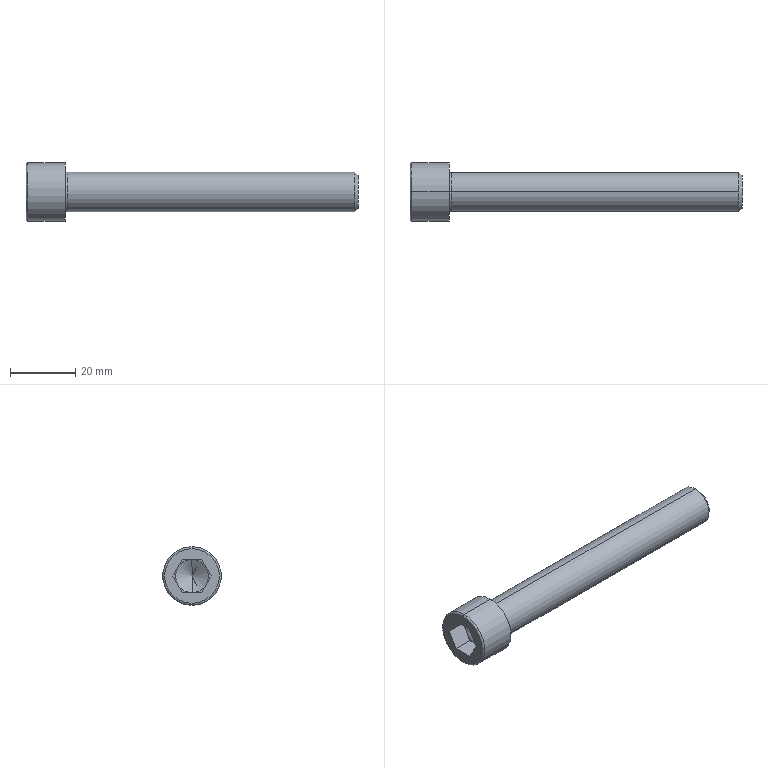Part | STEP file | socket head cap screw_bsi_BS EN ISO 4762 M12 x 90 - 36N | 1 solid | 27 faces | box 102 x 18 x 18 mm | volume 12605 mm3 | plane 15 | cone 4 | torus 4 | cylinder 4 | commonest cylinder face diameters 12 x2 18 x2